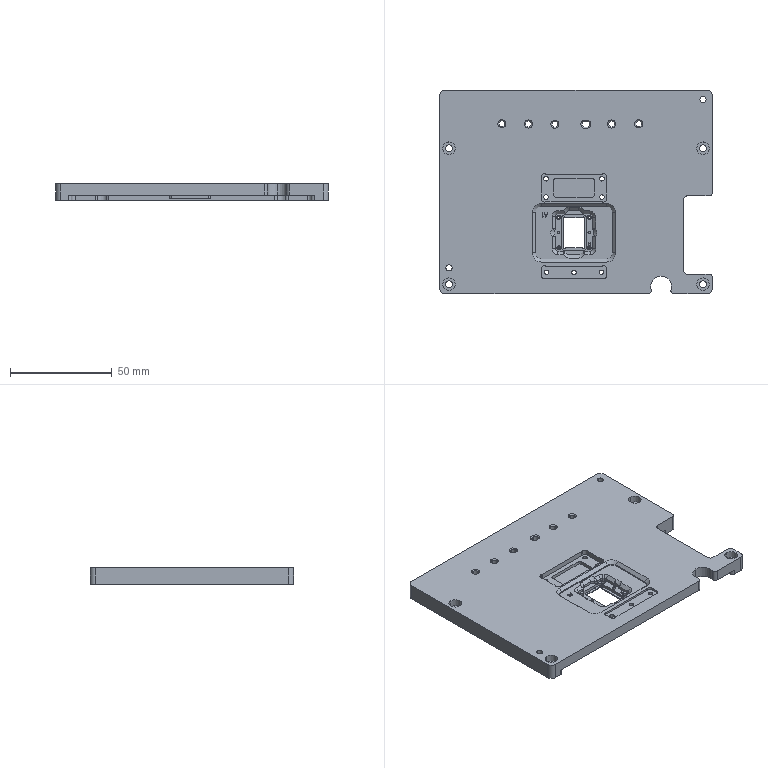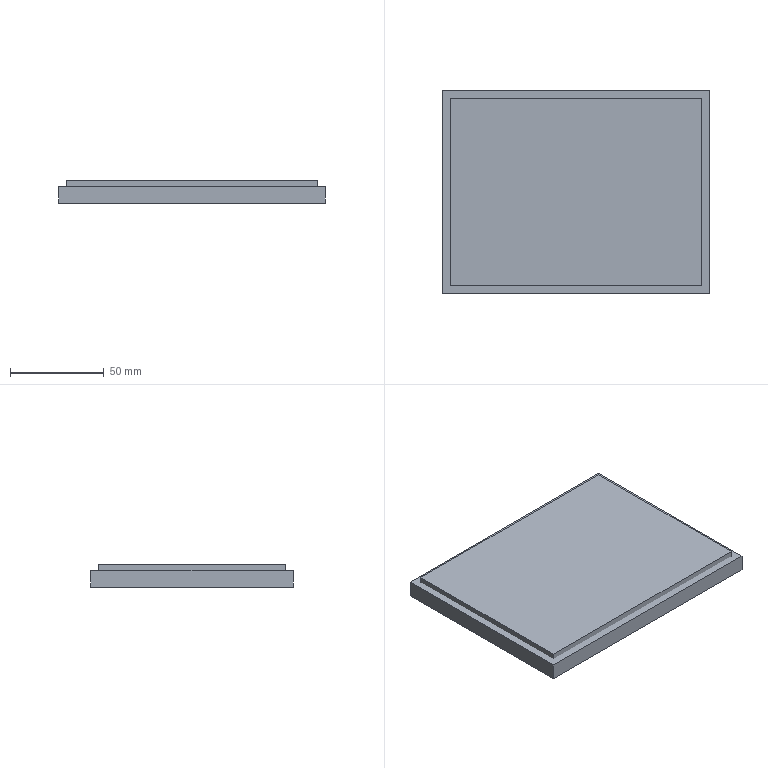CAM job | NX | 3-axis milling, drilling | part box 134 x 100 x 8 mm | stock box 142 x 108 x 12 mm
Tools:
number,name,description,diameter,corner_radius,flute_length,length,flutes
3,D63,Milling Tool-5 Parameters,63.0,0.0,50.0,75.0,2
1,D6A45,Milling Tool-5 Parameters,6.0,0.0,3.0,3.0,2
13,3.5ZT,Drilling Tool,3.5,0.0,35.0,50.0,2
12,2.2ZT,Drilling Tool,2.2,0.0,35.0,50.0,2
11,1.0ZT,Drilling Tool,1.0,0.0,35.0,50.0,2
23,3.0ZT,Drilling Tool,3.0,0.0,35.0,50.0,2
4,D10,Milling Tool-5 Parameters,10.0,0.0,50.0,75.0,2
16,D6JING,Milling Tool-5 Parameters,6.0,0.0,50.0,75.0,2
17,D4,Milling Tool-5 Parameters,4.0,0.0,50.0,75.0,2
18,D3,Milling Tool-5 Parameters,3.0,0.0,50.0,75.0,2
19,D2,Milling Tool-5 Parameters,2.0,0.0,50.0,75.0,2
19,D1.5,Milling Tool-5 Parameters,1.5,0.0,50.0,75.0,2
20,1.2ZT,Drilling Tool,1.2,0.0,35.0,50.0,2
24,D3A45,Milling Tool-5 Parameters,3.0,0.0,1.5,1.5,2
20,D1,Milling Tool-5 Parameters,1.0,0.0,50.0,75.0,2
Operations:
program,operation,operation_type,tool,method,geometry_group,spindle_rpm,surface_speed,feed_per_tooth,feed_cut,feed_plunge,cut_length_mm,path_length_mm,cut_time_min,machine_time_min
1,FLOOR_WALL_COPY,VolumeBased25DMillingOperation,D63,METHOD,A,6500.0,1286.0,0.0962,1250.0,100.0,709.799,763.799,0.5678,0.5732
1,DRILLING_COPY_1,Operation,D6A45,METHOD,A,5000.0,94.0,0.025,250.0,0.0,94.5,806.129,0.378,0.4492
1,DRILLING_COPY_1_COPY,Operation,3.5ZT,METHOD,A,2000.0,21.0,0.0375,150.0,0.0,54.206,436.375,0.3614,0.3996
1,DRILLING_COPY_1_COPY_COPY,Operation,2.2ZT,METHOD,A,2000.0,21.0,0.0375,150.0,0.0,97.01,534.562,0.6467,0.6905
1,DRILLING_COPY_1_COPY_COPY_COPY_2,Operation,3.0ZT,METHOD,A,2000.0,21.0,0.0375,150.0,0.0,54.507,249.499,0.3634,0.3829
1,DRILLING_COPY_1_COPY_COPY_COPY,Operation,1.0ZT,METHOD,A,3000.0,10.0,0.0167,100.0,0.0,47.602,210.095,0.476,0.4923
1,DRILLING_COPY_1_COPY_COPY_COPY_1,Operation,1.2ZT,METHOD,A,3000.0,11.0,0.0167,100.0,0.0,46.442,196.171,0.4644,0.4794
1,ADAPTIVE_MILLING_COPY,CavityMilling,D10,METHOD,A,9500.0,298.0,0.1842,3500.0,1000.0,3653.613,3797.713,1.045,1.06
1,CAVITY_MILL,CavityMilling,D10,METHOD,A,9500.0,298.0,0.1579,3000.0,1000.0,1426.383,1753.391,0.8765,0.9092
1,HOLE_MILLING,CylinderMilling,D6JING,METHOD,A,9500.0,179.0,0.1053,2000.0,100.0,234.406,301.906,0.1172,0.124
1,CAVITY_MILL_COPY,CavityMilling,D6JING,METHOD,A,9500.0,179.0,0.0947,1800.0,1000.0,2310.037,5855.11,1.631,1.985
1,ZLEVEL_PROFILE_COPY_COPY_COPY_1_COPY_COPY_1_COPY_COPY_COPY_1_COPY_COPY_COPY_1,ZLevelMilling,D4,METHOD,A,9500.0,89.0,0.0579,1100.0,1000.0,1493.207,4708.572,1.389,1.711
1,ZLEVEL_PROFILE_1_COPY_COPY_COPY_1,ZLevelMilling,D4,METHOD,A,9500.0,298.0,0.0526,1000.0,100.0,553.474,792.63,0.5535,0.5774
1,HOLE_MILLING_1,CylinderMilling,D4,METHOD,A,9500.0,119.0,0.0684,1300.0,100.0,410.43,921.222,0.3157,0.3668
1,ZLEVEL_PROFILE_COPY_COPY_COPY_1_COPY_COPY_1_COPY_COPY_COPY_1_COPY_COPY_COPY,ZLevelMilling,D3,METHOD,A,9500.0,89.0,0.0579,1100.0,1000.0,1222.661,4422.957,1.139,1.459
1,FLOOR_WALL,VolumeBased25DMillingOperation,D3,METHOD,A,9506.0,89.0,0.0526,1000.0,100.0,1459.751,1914.715,1.46,1.505
1,ZLEVEL_PROFILE_COPY_COPY_COPY_1_COPY_COPY_1_COPY_COPY_COPY_1_COPY_COPY,ZLevelMilling,D2,METHOD,A,9500.0,59.0,0.0526,1000.0,1000.0,226.651,289.151,0.2267,0.2329
1,HOLE_MILLING_COPY,CylinderMilling,D2,METHOD,A,9500.0,59.0,0.0526,1000.0,100.0,314.777,599.711,0.3148,0.3433
1,ZLEVEL_PROFILE_COPY_COPY_COPY_1_COPY_COPY_1_COPY_COPY_COPY_1_COPY_COPY_COPY_2,ZLevelMilling,D2,METHOD,A,9500.0,59.0,0.1053,2000.0,1000.0,3301.949,3360.449,1.666,1.672
1,ZLEVEL_PROFILE_COPY_COPY_COPY_1_COPY_COPY_1_COPY_COPY_COPY_1_COPY_COPY_COPY_2_COPY,ZLevelMilling,D2,METHOD,A,9500.0,59.0,0.1053,2000.0,1000.0,2001.85,2064.35,1.016,1.022
1,ZLEVEL_PROFILE_COPY_COPY_COPY_1_COPY_COPY_1_COPY_COPY_COPY_1_COPY_COPY_COPY_COPY_1,ZLevelMilling,D1.5,METHOD,A,9500.0,59.0,0.0526,1000.0,1000.0,921.723,5135.273,0.9217,1.343
1,HOLE_MILLING_1_COPY,CylinderMilling,D1.5,METHOD,A,9500.0,44.0,0.0421,800.0,100.0,105.769,431.969,0.1322,0.1648
1,11,ZLevelMilling,D6A45,METHOD,A,9500.0,179.0,0.0526,1000.0,100.0,886.671,2807.699,0.8867,1.079
1,11_COPY_COPY_COPY,ZLevelMilling,D3A45,METHOD,A,9500.0,179.0,0.0526,1000.0,100.0,99.595,463.323,0.0996,0.136
1,11_COPY_COPY_COPY_COPY,ZLevelMilling,D3A45,METHOD,A,9500.0,179.0,0.0526,1000.0,100.0,77.37,475.969,0.0774,0.1172
1,CUTTERCOMP19,CylinderMilling,D2,METHOD,A,9500.0,59.0,0.0421,800.0,100.0,39.151,324.085,0.0489,0.0774
2,FLOOR_WALL_COPY_COPY,VolumeBased25DMillingOperation,D63,METHOD,B,6500.0,1286.0,0.0962,1250.0,100.0,2711.196,3563.722,2.169,2.254
2,FLOOR_WALL_COPY_COPY_1,VolumeBased25DMillingOperation,D63,METHOD,B,6500.0,1286.0,0.0962,1250.0,100.0,677.799,731.799,0.5422,0.5476
2,CAVITY_MILL_1,CavityMilling,D10,METHOD,B,9500.0,298.0,0.1579,3000.0,1000.0,9070.96,9594.421,3.178,3.231
2,CAVITY_MILL_COPY_1,CavityMilling,D6JING,METHOD,B,9500.0,179.0,0.0947,1800.0,1000.0,271.225,1431.055,0.1805,0.2965
2,FLOOR_WALL_COPY_1,VolumeBased25DMillingOperation,D6JING,METHOD,B,9500.0,119.0,0.0658,1250.0,100.0,4099.329,4763.059,3.28,3.346
2,HOLE_MILLING_1_1,CylinderMilling,D3,METHOD,B,9500.0,89.0,0.0579,1100.0,100.0,290.305,867.341,0.2639,0.3216
2,ZLEVEL_PROFILE_COPY_COPY_COPY_1_COPY_COPY_1_COPY_COPY_COPY_1_COPY_COPY_1,ZLevelMilling,D3,METHOD,B,9500.0,89.0,0.0579,1100.0,1000.0,130.982,190.132,0.1221,0.128
2,ZLEVEL_PROFILE_COPY_COPY_COPY_1_COPY_COPY_1_COPY_COPY_COPY_1_COPY_COPY_1_COPY,ZLevelMilling,D1,METHOD,B,9500.0,44.0,0.0526,1000.0,1000.0,358.525,418.675,0.3585,0.3645
2,ZLEVEL_PROFILE_COPY_COPY_COPY_1_COPY_COPY_1_COPY_COPY_COPY_1_COPY_COPY_1_COPY_COPY,ZLevelMilling,D1,METHOD,B,9500.0,44.0,0.0526,1000.0,1000.0,137.911,277.769,0.1379,0.1519
2,11_COPY,ZLevelMilling,D6A45,METHOD,B,9500.0,179.0,0.0526,1000.0,100.0,698.365,1850.198,0.6984,0.8135
2,11_COPY_COPY,ZLevelMilling,D6A45,METHOD,B,9500.0,179.0,0.0526,1000.0,100.0,350.008,1762.322,0.35,0.4912
2,CUTTERCOMP20,ZLevelMilling,D1,METHOD,B,9500.0,44.0,0.0526,1000.0,1000.0,116.695,260.402,0.1167,0.1311